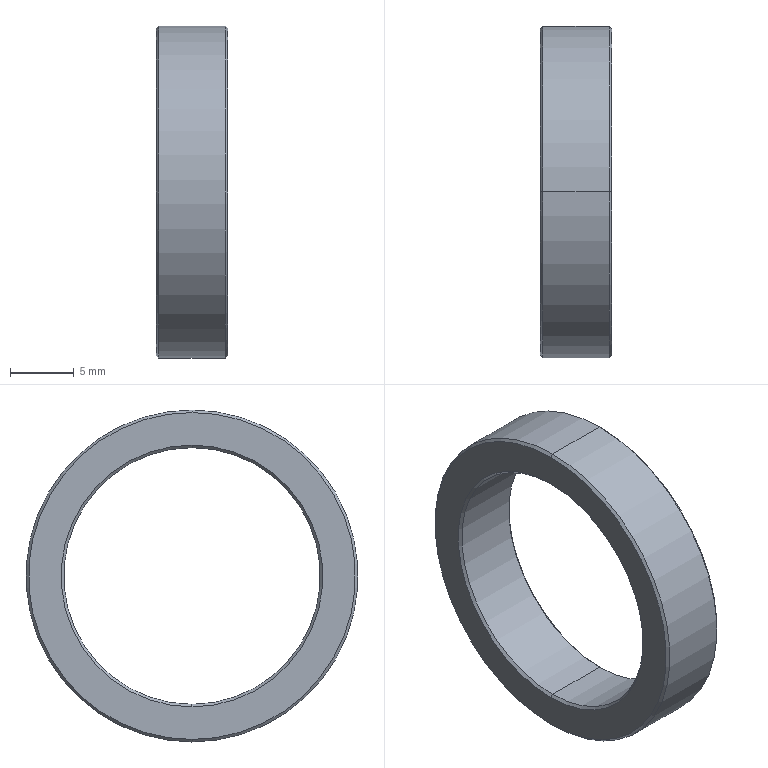Part | STEP file | 1 solid | 14 faces | box 5.6 x 26 x 26 mm | volume 1190 mm3 | cone 8 | cylinder 4 | plane 2 | commonest cylinder face diameters 20.1 x2 26 x2
STEP:
#1=CARTESIAN_POINT('',(0.,0.,0.));
#2=DIRECTION('',(0.,0.,1.));
#3=DIRECTION('',(1.,0.,0.));
#4=AXIS2_PLACEMENT_3D('',#1,#2,#3);
#5=CARTESIAN_POINT('',(0.2,0.,10.05));
#6=VERTEX_POINT('',#5);
#7=CARTESIAN_POINT('',(0.,0.,10.25));
#8=VERTEX_POINT('',#7);
#9=CARTESIAN_POINT('',(0.2,0.,10.05));
#10=DIRECTION('',(-0.7071,0.,0.7071));
#11=VECTOR('',#10,1.);
#12=LINE('',#9,#11);
#13=CARTESIAN_POINT('',(0.2,0.,0.));
#14=DIRECTION('',(-1.,0.,0.));
#15=DIRECTION('',(0.,0.,1.));
#16=AXIS2_PLACEMENT_3D('',#13,#14,#15);
#17=CONICAL_SURFACE('',#16,10.05,0.7854);
#18=CARTESIAN_POINT('',(6.283,0.));
#19=DIRECTION('',(0.,1.));
#20=VECTOR('',#19,1.);
#21=LINE('',#18,#20);
#22=(GEOMETRIC_REPRESENTATION_CONTEXT(2)PARAMETRIC_REPRESENTATION_CONTEXT()REPRESENTATION_CONTEXT('',''));
#23=DEFINITIONAL_REPRESENTATION('',(#21),#22);
#24=PCURVE('',#17,#23);
#25=CARTESIAN_POINT('',(0.2,0.,0.));
#26=DIRECTION('',(-1.,0.,0.));
#27=DIRECTION('',(0.,0.,1.));
#28=AXIS2_PLACEMENT_3D('',#25,#26,#27);
#29=CONICAL_SURFACE('',#28,10.05,0.7854);
#30=CARTESIAN_POINT('',(0.,0.));
#31=DIRECTION('',(0.,1.));
#32=VECTOR('',#31,1.);
#33=LINE('',#30,#32);
#34=(GEOMETRIC_REPRESENTATION_CONTEXT(2)PARAMETRIC_REPRESENTATION_CONTEXT()REPRESENTATION_CONTEXT('',''));
#35=DEFINITIONAL_REPRESENTATION('',(#33),#34);
#36=PCURVE('',#29,#35);
#37=SURFACE_CURVE('',#12,(#24,#36),.PCURVE_S1.);
#38=EDGE_CURVE('',#6,#8,#37,.T.);
#39=ORIENTED_EDGE('',*,*,#38,.T.);
#40=CARTESIAN_POINT('',(0.,0.,-10.25));
#41=VERTEX_POINT('',#40);
#42=CARTESIAN_POINT('',(0.,0.,0.));
#43=DIRECTION('',(1.,0.,0.));
#44=DIRECTION('',(0.,0.,-1.));
#45=AXIS2_PLACEMENT_3D('',#42,#43,#44);
#46=CIRCLE('',#45,10.25);
#47=CARTESIAN_POINT('',(9.425,0.2));
#48=DIRECTION('',(-1.,0.));
#49=VECTOR('',#48,1.);
#50=LINE('',#47,#49);
#51=(GEOMETRIC_REPRESENTATION_CONTEXT(2)PARAMETRIC_REPRESENTATION_CONTEXT()REPRESENTATION_CONTEXT('',''));
#52=DEFINITIONAL_REPRESENTATION('',(#50),#51);
#53=PCURVE('',#17,#52);
#54=CARTESIAN_POINT('',(0.,13.,0.));
#55=DIRECTION('',(1.,0.,0.));
#56=DIRECTION('',(0.,0.,-1.));
#57=AXIS2_PLACEMENT_3D('',#54,#55,#56);
#58=PLANE('',#57);
#59=CARTESIAN_POINT('',(0.,-13.));
#60=DIRECTION('',(1.,0.));
#61=AXIS2_PLACEMENT_2D('',#59,#60);
#62=CIRCLE('',#61,10.25);
#63=(GEOMETRIC_REPRESENTATION_CONTEXT(2)PARAMETRIC_REPRESENTATION_CONTEXT()REPRESENTATION_CONTEXT('',''));
#64=DEFINITIONAL_REPRESENTATION('',(#62),#63);
#65=PCURVE('',#58,#64);
#66=SURFACE_CURVE('',#46,(#53,#65),.PCURVE_S1.);
#67=EDGE_CURVE('',#8,#41,#66,.T.);
#68=ORIENTED_EDGE('',*,*,#67,.T.);
#69=CARTESIAN_POINT('',(0.2,0.,-10.05));
#70=VERTEX_POINT('',#69);
#71=CARTESIAN_POINT('',(0.2,0.,-10.05));
#72=DIRECTION('',(-0.7071,0.,-0.7071));
#73=VECTOR('',#72,1.);
#74=LINE('',#71,#73);
#75=CARTESIAN_POINT('',(3.142,0.));
#76=DIRECTION('',(0.,1.));
#77=VECTOR('',#76,1.);
#78=LINE('',#75,#77);
#79=(GEOMETRIC_REPRESENTATION_CONTEXT(2)PARAMETRIC_REPRESENTATION_CONTEXT()REPRESENTATION_CONTEXT('',''));
#80=DEFINITIONAL_REPRESENTATION('',(#78),#79);
#81=PCURVE('',#17,#80);
#82=CARTESIAN_POINT('',(3.142,0.));
#83=DIRECTION('',(0.,1.));
#84=VECTOR('',#83,1.);
#85=LINE('',#82,#84);
#86=(GEOMETRIC_REPRESENTATION_CONTEXT(2)PARAMETRIC_REPRESENTATION_CONTEXT()REPRESENTATION_CONTEXT('',''));
#87=DEFINITIONAL_REPRESENTATION('',(#85),#86);
#88=PCURVE('',#29,#87);
#89=SURFACE_CURVE('',#74,(#81,#88),.PCURVE_S1.);
#90=EDGE_CURVE('',#70,#41,#89,.T.);
#91=ORIENTED_EDGE('',*,*,#90,.F.);
#92=CARTESIAN_POINT('',(0.2,0.,0.));
#93=DIRECTION('',(-1.,0.,0.));
#94=DIRECTION('',(0.,0.,-1.));
#95=AXIS2_PLACEMENT_3D('',#92,#93,#94);
#96=CIRCLE('',#95,10.05);
#97=CARTESIAN_POINT('',(3.142,0.));
#98=DIRECTION('',(1.,0.));
#99=VECTOR('',#98,1.);
#100=LINE('',#97,#99);
#101=(GEOMETRIC_REPRESENTATION_CONTEXT(2)PARAMETRIC_REPRESENTATION_CONTEXT()REPRESENTATION_CONTEXT('',''));
#102=DEFINITIONAL_REPRESENTATION('',(#100),#101);
#103=PCURVE('',#17,#102);
#104=CARTESIAN_POINT('',(0.,0.,0.));
#105=DIRECTION('',(-1.,0.,0.));
#106=DIRECTION('',(0.,0.,1.));
#107=AXIS2_PLACEMENT_3D('',#104,#105,#106);
#108=CYLINDRICAL_SURFACE('',#107,10.05);
#109=CARTESIAN_POINT('',(3.142,-0.2));
#110=DIRECTION('',(1.,0.));
#111=VECTOR('',#110,1.);
#112=LINE('',#109,#111);
#113=(GEOMETRIC_REPRESENTATION_CONTEXT(2)PARAMETRIC_REPRESENTATION_CONTEXT()REPRESENTATION_CONTEXT('',''));
#114=DEFINITIONAL_REPRESENTATION('',(#112),#113);
#115=PCURVE('',#108,#114);
#116=SURFACE_CURVE('',#96,(#103,#115),.PCURVE_S1.);
#117=EDGE_CURVE('',#70,#6,#116,.T.);
#118=ORIENTED_EDGE('',*,*,#117,.T.);
#119=EDGE_LOOP('',(#39,#68,#91,#118));
#120=FACE_BOUND('',#119,.F.);
#121=ADVANCED_FACE('',(#120),#17,.F.);
#122=CARTESIAN_POINT('',(0.,0.,12.8));
#123=VERTEX_POINT('',#122);
#124=CARTESIAN_POINT('',(0.,0.,-12.8));
#125=VERTEX_POINT('',#124);
#126=CARTESIAN_POINT('',(0.,0.,0.));
#127=DIRECTION('',(-1.,0.,0.));
#128=DIRECTION('',(0.,0.,-1.));
#129=AXIS2_PLACEMENT_3D('',#126,#127,#128);
#130=CIRCLE('',#129,12.8);
#131=CARTESIAN_POINT('',(0.,0.,0.));
#132=DIRECTION('',(1.,0.,0.));
#133=DIRECTION('',(0.,0.,-1.));
#134=AXIS2_PLACEMENT_3D('',#131,#132,#133);
#135=CONICAL_SURFACE('',#134,12.8,0.7854);
#136=CARTESIAN_POINT('',(6.283,0.));
#137=DIRECTION('',(-1.,0.));
#138=VECTOR('',#137,1.);
#139=LINE('',#136,#138);
#140=(GEOMETRIC_REPRESENTATION_CONTEXT(2)PARAMETRIC_REPRESENTATION_CONTEXT()REPRESENTATION_CONTEXT('',''));
#141=DEFINITIONAL_REPRESENTATION('',(#139),#140);
#142=PCURVE('',#135,#141);
#143=CARTESIAN_POINT('',(12.8,-13.));
#144=CARTESIAN_POINT('',(12.8,-35.17));
#145=CARTESIAN_POINT('',(-6.4,-24.085));
#146=CARTESIAN_POINT('',(-25.6,-13.));
#147=CARTESIAN_POINT('',(-6.4,-1.915));
#148=CARTESIAN_POINT('',(12.8,9.17));
#149=CARTESIAN_POINT('',(12.8,-13.));
#150=(BOUNDED_CURVE()B_SPLINE_CURVE(2,(#143,#144,#145,#146,#147,#148,#149),.UNSPECIFIED.,.T.,.F.)B_SPLINE_CURVE_WITH_KNOTS((1,2,2,2,2,1),(-2.094,0.,2.094,4.189,6.283,8.378),.UNSPECIFIED.)CURVE()GEOMETRIC_REPRESENTATION_ITEM()RATIONAL_B_SPLINE_CURVE((1.,0.5,1.,0.5,1.,0.5,1.))REPRESENTATION_ITEM(''));
#151=(GEOMETRIC_REPRESENTATION_CONTEXT(2)PARAMETRIC_REPRESENTATION_CONTEXT()REPRESENTATION_CONTEXT('',''));
#152=DEFINITIONAL_REPRESENTATION('',(#150),#151);
#153=PCURVE('',#58,#152);
#154=SURFACE_CURVE('',#130,(#142,#153),.PCURVE_S1.);
#155=EDGE_CURVE('',#123,#125,#154,.T.);
#156=ORIENTED_EDGE('',*,*,#155,.F.);
#157=CARTESIAN_POINT('',(0.2,0.,13.));
#158=VERTEX_POINT('',#157);
#159=CARTESIAN_POINT('',(0.,0.,12.8));
#160=DIRECTION('',(0.7071,0.,0.7071));
#161=VECTOR('',#160,1.);
#162=LINE('',#159,#161);
#163=CARTESIAN_POINT('',(3.142,0.));
#164=DIRECTION('',(0.,1.));
#165=VECTOR('',#164,1.);
#166=LINE('',#163,#165);
#167=(GEOMETRIC_REPRESENTATION_CONTEXT(2)PARAMETRIC_REPRESENTATION_CONTEXT()REPRESENTATION_CONTEXT('',''));
#168=DEFINITIONAL_REPRESENTATION('',(#166),#167);
#169=PCURVE('',#135,#168);
#170=CARTESIAN_POINT('',(0.,0.,0.));
#171=DIRECTION('',(1.,0.,0.));
#172=DIRECTION('',(0.,0.,-1.));
#173=AXIS2_PLACEMENT_3D('',#170,#171,#172);
#174=CONICAL_SURFACE('',#173,12.8,0.7854);
#175=CARTESIAN_POINT('',(3.142,0.));
#176=DIRECTION('',(0.,1.));
#177=VECTOR('',#176,1.);
#178=LINE('',#175,#177);
#179=(GEOMETRIC_REPRESENTATION_CONTEXT(2)PARAMETRIC_REPRESENTATION_CONTEXT()REPRESENTATION_CONTEXT('',''));
#180=DEFINITIONAL_REPRESENTATION('',(#178),#179);
#181=PCURVE('',#174,#180);
#182=SURFACE_CURVE('',#162,(#169,#181),.PCURVE_S1.);
#183=EDGE_CURVE('',#123,#158,#182,.T.);
#184=ORIENTED_EDGE('',*,*,#183,.T.);
#185=CARTESIAN_POINT('',(0.2,0.,-13.));
#186=VERTEX_POINT('',#185);
#187=CARTESIAN_POINT('',(0.2,0.,0.));
#188=DIRECTION('',(1.,0.,0.));
#189=DIRECTION('',(0.,0.,-1.));
#190=AXIS2_PLACEMENT_3D('',#187,#188,#189);
#191=CIRCLE('',#190,13.);
#192=CARTESIAN_POINT('',(0.,0.2));
#193=DIRECTION('',(1.,0.));
#194=VECTOR('',#193,1.);
#195=LINE('',#192,#194);
#196=(GEOMETRIC_REPRESENTATION_CONTEXT(2)PARAMETRIC_REPRESENTATION_CONTEXT()REPRESENTATION_CONTEXT('',''));
#197=DEFINITIONAL_REPRESENTATION('',(#195),#196);
#198=PCURVE('',#135,#197);
#199=CARTESIAN_POINT('',(0.,0.,0.));
#200=DIRECTION('',(-1.,0.,0.));
#201=DIRECTION('',(0.,0.,1.));
#202=AXIS2_PLACEMENT_3D('',#199,#200,#201);
#203=CYLINDRICAL_SURFACE('',#202,13.);
#204=CARTESIAN_POINT('',(3.142,-0.2));
#205=DIRECTION('',(-1.,0.));
#206=VECTOR('',#205,1.);
#207=LINE('',#204,#206);
#208=(GEOMETRIC_REPRESENTATION_CONTEXT(2)PARAMETRIC_REPRESENTATION_CONTEXT()REPRESENTATION_CONTEXT('',''));
#209=DEFINITIONAL_REPRESENTATION('',(#207),#208);
#210=PCURVE('',#203,#209);
#211=SURFACE_CURVE('',#191,(#198,#210),.PCURVE_S1.);
#212=EDGE_CURVE('',#186,#158,#211,.T.);
#213=ORIENTED_EDGE('',*,*,#212,.F.);
#214=CARTESIAN_POINT('',(0.,0.,-12.8));
#215=DIRECTION('',(0.7071,0.,-0.7071));
#216=VECTOR('',#215,1.);
#217=LINE('',#214,#216);
#218=CARTESIAN_POINT('',(0.,0.));
#219=DIRECTION('',(0.,1.));
#220=VECTOR('',#219,1.);
#221=LINE('',#218,#220);
#222=(GEOMETRIC_REPRESENTATION_CONTEXT(2)PARAMETRIC_REPRESENTATION_CONTEXT()REPRESENTATION_CONTEXT('',''));
#223=DEFINITIONAL_REPRESENTATION('',(#221),#222);
#224=PCURVE('',#135,#223);
#225=CARTESIAN_POINT('',(6.283,0.));
#226=DIRECTION('',(0.,1.));
#227=VECTOR('',#226,1.);
#228=LINE('',#225,#227);
#229=(GEOMETRIC_REPRESENTATION_CONTEXT(2)PARAMETRIC_REPRESENTATION_CONTEXT()REPRESENTATION_CONTEXT('',''));
#230=DEFINITIONAL_REPRESENTATION('',(#228),#229);
#231=PCURVE('',#174,#230);
#232=SURFACE_CURVE('',#217,(#224,#231),.PCURVE_S1.);
#233=EDGE_CURVE('',#125,#186,#232,.T.);
#234=ORIENTED_EDGE('',*,*,#233,.F.);
#235=EDGE_LOOP('',(#156,#184,#213,#234));
#236=FACE_BOUND('',#235,.T.);
#237=ADVANCED_FACE('',(#236),#135,.T.);
#238=CARTESIAN_POINT('',(5.6,0.,-12.8));
#239=VERTEX_POINT('',#238);
#240=CARTESIAN_POINT('',(5.6,0.,12.8));
#241=VERTEX_POINT('',#240);
#242=CARTESIAN_POINT('',(5.6,0.,0.));
#243=DIRECTION('',(1.,0.,0.));
#244=DIRECTION('',(0.,0.,1.));
#245=AXIS2_PLACEMENT_3D('',#242,#243,#244);
#246=CIRCLE('',#245,12.8);
#247=CARTESIAN_POINT('',(5.4,0.,0.));
#248=DIRECTION('',(-1.,0.,0.));
#249=DIRECTION('',(0.,0.,1.));
#250=AXIS2_PLACEMENT_3D('',#247,#248,#249);
#251=CONICAL_SURFACE('',#250,13.,0.7854);
#252=CARTESIAN_POINT('',(6.283,-0.2));
#253=DIRECTION('',(-1.,0.));
#254=VECTOR('',#253,1.);
#255=LINE('',#252,#254);
#256=(GEOMETRIC_REPRESENTATION_CONTEXT(2)PARAMETRIC_REPRESENTATION_CONTEXT()REPRESENTATION_CONTEXT('',''));
#257=DEFINITIONAL_REPRESENTATION('',(#255),#256);
#258=PCURVE('',#251,#257);
#259=CARTESIAN_POINT('',(5.6,13.,0.));
#260=DIRECTION('',(-1.,0.,0.));
#261=DIRECTION('',(0.,0.,1.));
#262=AXIS2_PLACEMENT_3D('',#259,#260,#261);
#263=PLANE('',#262);
#264=CARTESIAN_POINT('',(12.8,-13.));
#265=CARTESIAN_POINT('',(12.8,-35.17));
#266=CARTESIAN_POINT('',(-6.4,-24.085));
#267=CARTESIAN_POINT('',(-25.6,-13.));
#268=CARTESIAN_POINT('',(-6.4,-1.915));
#269=CARTESIAN_POINT('',(12.8,9.17));
#270=CARTESIAN_POINT('',(12.8,-13.));
#271=(BOUNDED_CURVE()B_SPLINE_CURVE(2,(#264,#265,#266,#267,#268,#269,#270),.UNSPECIFIED.,.T.,.F.)B_SPLINE_CURVE_WITH_KNOTS((1,2,2,2,2,1),(-2.094,0.,2.094,4.189,6.283,8.378),.UNSPECIFIED.)CURVE()GEOMETRIC_REPRESENTATION_ITEM()RATIONAL_B_SPLINE_CURVE((1.,0.5,1.,0.5,1.,0.5,1.))REPRESENTATION_ITEM(''));
#272=(GEOMETRIC_REPRESENTATION_CONTEXT(2)PARAMETRIC_REPRESENTATION_CONTEXT()REPRESENTATION_CONTEXT('',''));
#273=DEFINITIONAL_REPRESENTATION('',(#271),#272);
#274=PCURVE('',#263,#273);
#275=SURFACE_CURVE('',#246,(#258,#274),.PCURVE_S1.);
#276=EDGE_CURVE('',#239,#241,#275,.T.);
#277=ORIENTED_EDGE('',*,*,#276,.F.);
#278=CARTESIAN_POINT('',(5.4,0.,-13.));
#279=VERTEX_POINT('',#278);
#280=CARTESIAN_POINT('',(5.4,0.,-13.));
#281=DIRECTION('',(-0.7071,0.,-0.7071));
#282=VECTOR('',#281,1.);
#283=LINE('',#280,#282);
#284=CARTESIAN_POINT('',(3.142,0.));
#285=DIRECTION('',(0.,1.));
#286=VECTOR('',#285,1.);
#287=LINE('',#284,#286);
#288=(GEOMETRIC_REPRESENTATION_CONTEXT(2)PARAMETRIC_REPRESENTATION_CONTEXT()REPRESENTATION_CONTEXT('',''));
#289=DEFINITIONAL_REPRESENTATION('',(#287),#288);
#290=PCURVE('',#251,#289);
#291=CARTESIAN_POINT('',(5.4,0.,0.));
#292=DIRECTION('',(-1.,0.,0.));
#293=DIRECTION('',(0.,0.,1.));
#294=AXIS2_PLACEMENT_3D('',#291,#292,#293);
#295=CONICAL_SURFACE('',#294,13.,0.7854);
#296=CARTESIAN_POINT('',(3.142,0.));
#297=DIRECTION('',(0.,1.));
#298=VECTOR('',#297,1.);
#299=LINE('',#296,#298);
#300=(GEOMETRIC_REPRESENTATION_CONTEXT(2)PARAMETRIC_REPRESENTATION_CONTEXT()REPRESENTATION_CONTEXT('',''));
#301=DEFINITIONAL_REPRESENTATION('',(#299),#300);
#302=PCURVE('',#295,#301);
#303=SURFACE_CURVE('',#283,(#290,#302),.PCURVE_S1.);
#304=EDGE_CURVE('',#239,#279,#303,.T.);
#305=ORIENTED_EDGE('',*,*,#304,.T.);
#306=CARTESIAN_POINT('',(5.4,0.,13.));
#307=VERTEX_POINT('',#306);
#308=CARTESIAN_POINT('',(5.4,0.,0.));
#309=DIRECTION('',(-1.,0.,0.));
#310=DIRECTION('',(0.,0.,1.));
#311=AXIS2_PLACEMENT_3D('',#308,#309,#310);
#312=CIRCLE('',#311,13.);
#313=CARTESIAN_POINT('',(0.,0.));
#314=DIRECTION('',(1.,0.));
#315=VECTOR('',#314,1.);
#316=LINE('',#313,#315);
#317=(GEOMETRIC_REPRESENTATION_CONTEXT(2)PARAMETRIC_REPRESENTATION_CONTEXT()REPRESENTATION_CONTEXT('',''));
#318=DEFINITIONAL_REPRESENTATION('',(#316),#317);
#319=PCURVE('',#251,#318);
#320=CARTESIAN_POINT('',(0.,-5.4));
#321=DIRECTION('',(1.,0.));
#322=VECTOR('',#321,1.);
#323=LINE('',#320,#322);
#324=(GEOMETRIC_REPRESENTATION_CONTEXT(2)PARAMETRIC_REPRESENTATION_CONTEXT()REPRESENTATION_CONTEXT('',''));
#325=DEFINITIONAL_REPRESENTATION('',(#323),#324);
#326=PCURVE('',#203,#325);
#327=SURFACE_CURVE('',#312,(#319,#326),.PCURVE_S1.);
#328=EDGE_CURVE('',#307,#279,#327,.T.);
#329=ORIENTED_EDGE('',*,*,#328,.F.);
#330=CARTESIAN_POINT('',(5.4,0.,13.));
#331=DIRECTION('',(-0.7071,0.,0.7071));
#332=VECTOR('',#331,1.);
#333=LINE('',#330,#332);
#334=CARTESIAN_POINT('',(0.,0.));
#335=DIRECTION('',(0.,1.));
#336=VECTOR('',#335,1.);
#337=LINE('',#334,#336);
#338=(GEOMETRIC_REPRESENTATION_CONTEXT(2)PARAMETRIC_REPRESENTATION_CONTEXT()REPRESENTATION_CONTEXT('',''));
#339=DEFINITIONAL_REPRESENTATION('',(#337),#338);
#340=PCURVE('',#251,#339);
#341=CARTESIAN_POINT('',(6.283,0.));
#342=DIRECTION('',(0.,1.));
#343=VECTOR('',#342,1.);
#344=LINE('',#341,#343);
#345=(GEOMETRIC_REPRESENTATION_CONTEXT(2)PARAMETRIC_REPRESENTATION_CONTEXT()REPRESENTATION_CONTEXT('',''));
#346=DEFINITIONAL_REPRESENTATION('',(#344),#345);
#347=PCURVE('',#295,#346);
#348=SURFACE_CURVE('',#333,(#340,#347),.PCURVE_S1.);
#349=EDGE_CURVE('',#241,#307,#348,.T.);
#350=ORIENTED_EDGE('',*,*,#349,.F.);
#351=EDGE_LOOP('',(#277,#305,#329,#350));
#352=FACE_BOUND('',#351,.T.);
#353=ADVANCED_FACE('',(#352),#251,.T.);
#354=CARTESIAN_POINT('',(5.4,0.,-10.05));
#355=VERTEX_POINT('',#354);
#356=CARTESIAN_POINT('',(5.6,0.,-10.25));
#357=VERTEX_POINT('',#356);
#358=CARTESIAN_POINT('',(5.6,0.,-10.25));
#359=DIRECTION('',(0.7071,0.,-0.7071));
#360=VECTOR('',#359,1.);
#361=LINE('',#358,#360);
#362=CARTESIAN_POINT('',(5.6,0.,0.));
#363=DIRECTION('',(1.,0.,0.));
#364=DIRECTION('',(0.,0.,-1.));
#365=AXIS2_PLACEMENT_3D('',#362,#363,#364);
#366=CONICAL_SURFACE('',#365,10.25,0.7854);
#367=CARTESIAN_POINT('',(6.283,0.));
#368=DIRECTION('',(0.,1.));
#369=VECTOR('',#368,1.);
#370=LINE('',#367,#369);
#371=(GEOMETRIC_REPRESENTATION_CONTEXT(2)PARAMETRIC_REPRESENTATION_CONTEXT()REPRESENTATION_CONTEXT('',''));
#372=DEFINITIONAL_REPRESENTATION('',(#370),#371);
#373=PCURVE('',#366,#372);
#374=CARTESIAN_POINT('',(5.6,0.,0.));
#375=DIRECTION('',(1.,0.,0.));
#376=DIRECTION('',(0.,0.,-1.));
#377=AXIS2_PLACEMENT_3D('',#374,#375,#376);
#378=CONICAL_SURFACE('',#377,10.25,0.7854);
#379=CARTESIAN_POINT('',(0.,0.));
#380=DIRECTION('',(0.,1.));
#381=VECTOR('',#380,1.);
#382=LINE('',#379,#381);
#383=(GEOMETRIC_REPRESENTATION_CONTEXT(2)PARAMETRIC_REPRESENTATION_CONTEXT()REPRESENTATION_CONTEXT('',''));
#384=DEFINITIONAL_REPRESENTATION('',(#382),#383);
#385=PCURVE('',#378,#384);
#386=SURFACE_CURVE('',#361,(#373,#385),.PCURVE_S1.);
#387=EDGE_CURVE('',#355,#357,#386,.T.);
#388=ORIENTED_EDGE('',*,*,#387,.T.);
#389=CARTESIAN_POINT('',(5.6,0.,10.25));
#390=VERTEX_POINT('',#389);
#391=CARTESIAN_POINT('',(5.6,0.,0.));
#392=DIRECTION('',(-1.,0.,0.));
#393=DIRECTION('',(0.,0.,1.));
#394=AXIS2_PLACEMENT_3D('',#391,#392,#393);
#395=CIRCLE('',#394,10.25);
#396=CARTESIAN_POINT('',(9.425,0.));
#397=DIRECTION('',(-1.,0.));
#398=VECTOR('',#397,1.);
#399=LINE('',#396,#398);
#400=(GEOMETRIC_REPRESENTATION_CONTEXT(2)PARAMETRIC_REPRESENTATION_CONTEXT()REPRESENTATION_CONTEXT('',''));
#401=DEFINITIONAL_REPRESENTATION('',(#399),#400);
#402=PCURVE('',#366,#401);
#403=CARTESIAN_POINT('',(0.,-13.));
#404=DIRECTION('',(1.,0.));
#405=AXIS2_PLACEMENT_2D('',#403,#404);
#406=CIRCLE('',#405,10.25);
#407=(GEOMETRIC_REPRESENTATION_CONTEXT(2)PARAMETRIC_REPRESENTATION_CONTEXT()REPRESENTATION_CONTEXT('',''));
#408=DEFINITIONAL_REPRESENTATION('',(#406),#407);
#409=PCURVE('',#263,#408);
#410=SURFACE_CURVE('',#395,(#402,#409),.PCURVE_S1.);
#411=EDGE_CURVE('',#357,#390,#410,.T.);
#412=ORIENTED_EDGE('',*,*,#411,.T.);
#413=CARTESIAN_POINT('',(5.4,0.,10.05));
#414=VERTEX_POINT('',#413);
#415=CARTESIAN_POINT('',(5.6,0.,10.25));
#416=DIRECTION('',(0.7071,0.,0.7071));
#417=VECTOR('',#416,1.);
#418=LINE('',#415,#417);
#419=CARTESIAN_POINT('',(3.142,0.));
#420=DIRECTION('',(0.,1.));
#421=VECTOR('',#420,1.);
#422=LINE('',#419,#421);
#423=(GEOMETRIC_REPRESENTATION_CONTEXT(2)PARAMETRIC_REPRESENTATION_CONTEXT()REPRESENTATION_CONTEXT('',''));
#424=DEFINITIONAL_REPRESENTATION('',(#422),#423);
#425=PCURVE('',#366,#424);
#426=CARTESIAN_POINT('',(3.142,0.));
#427=DIRECTION('',(0.,1.));
#428=VECTOR('',#427,1.);
#429=LINE('',#426,#428);
#430=(GEOMETRIC_REPRESENTATION_CONTEXT(2)PARAMETRIC_REPRESENTATION_CONTEXT()REPRESENTATION_CONTEXT('',''));
#431=DEFINITIONAL_REPRESENTATION('',(#429),#430);
#432=PCURVE('',#378,#431);
#433=SURFACE_CURVE('',#418,(#425,#432),.PCURVE_S1.);
#434=EDGE_CURVE('',#414,#390,#433,.T.);
#435=ORIENTED_EDGE('',*,*,#434,.F.);
#436=CARTESIAN_POINT('',(5.4,0.,0.));
#437=DIRECTION('',(1.,0.,0.));
#438=DIRECTION('',(0.,0.,1.));
#439=AXIS2_PLACEMENT_3D('',#436,#437,#438);
#440=CIRCLE('',#439,10.05);
#441=CARTESIAN_POINT('',(3.142,-0.2));
#442=DIRECTION('',(1.,0.));
#443=VECTOR('',#442,1.);
#444=LINE('',#441,#443);
#445=(GEOMETRIC_REPRESENTATION_CONTEXT(2)PARAMETRIC_REPRESENTATION_CONTEXT()REPRESENTATION_CONTEXT('',''));
#446=DEFINITIONAL_REPRESENTATION('',(#444),#445);
#447=PCURVE('',#366,#446);
#448=CARTESIAN_POINT('',(6.283,-5.4));
#449=DIRECTION('',(-1.,0.));
#450=VECTOR('',#449,1.);
#451=LINE('',#448,#450);
#452=(GEOMETRIC_REPRESENTATION_CONTEXT(2)PARAMETRIC_REPRESENTATION_CONTEXT()REPRESENTATION_CONTEXT('',''));
#453=DEFINITIONAL_REPRESENTATION('',(#451),#452);
#454=PCURVE('',#108,#453);
#455=SURFACE_CURVE('',#440,(#447,#454),.PCURVE_S1.);
#456=EDGE_CURVE('',#414,#355,#455,.T.);
#457=ORIENTED_EDGE('',*,*,#456,.T.);
#458=EDGE_LOOP('',(#388,#412,#435,#457));
#459=FACE_BOUND('',#458,.F.);
#460=ADVANCED_FACE('',(#459),#366,.F.);
#461=ORIENTED_EDGE('',*,*,#328,.T.);
#462=CARTESIAN_POINT('',(0.,0.,-13.));
#463=DIRECTION('',(-1.,0.,0.));
#464=VECTOR('',#463,1.);
#465=LINE('',#462,#464);
#466=CARTESIAN_POINT('',(3.142,0.));
#467=DIRECTION('',(0.,1.));
#468=VECTOR('',#467,1.);
#469=LINE('',#466,#468);
#470=(GEOMETRIC_REPRESENTATION_CONTEXT(2)PARAMETRIC_REPRESENTATION_CONTEXT()REPRESENTATION_CONTEXT('',''));
#471=DEFINITIONAL_REPRESENTATION('',(#469),#470);
#472=PCURVE('',#203,#471);
#473=CARTESIAN_POINT('',(0.,0.,0.));
#474=DIRECTION('',(-1.,0.,0.));
#475=DIRECTION('',(0.,0.,1.));
#476=AXIS2_PLACEMENT_3D('',#473,#474,#475);
#477=CYLINDRICAL_SURFACE('',#476,13.);
#478=CARTESIAN_POINT('',(3.142,0.));
#479=DIRECTION('',(0.,1.));
#480=VECTOR('',#479,1.);
#481=LINE('',#478,#480);
#482=(GEOMETRIC_REPRESENTATION_CONTEXT(2)PARAMETRIC_REPRESENTATION_CONTEXT()REPRESENTATION_CONTEXT('',''));
#483=DEFINITIONAL_REPRESENTATION('',(#481),#482);
#484=PCURVE('',#477,#483);
#485=SURFACE_CURVE('',#465,(#472,#484),.PCURVE_S1.);
#486=EDGE_CURVE('',#279,#186,#485,.T.);
#487=ORIENTED_EDGE('',*,*,#486,.T.);
#488=ORIENTED_EDGE('',*,*,#212,.T.);
#489=CARTESIAN_POINT('',(0.,0.,13.));
#490=DIRECTION('',(-1.,0.,0.));
#491=VECTOR('',#490,1.);
#492=LINE('',#489,#491);
#493=CARTESIAN_POINT('',(0.,0.));
#494=DIRECTION('',(0.,1.));
#495=VECTOR('',#494,1.);
#496=LINE('',#493,#495);
#497=(GEOMETRIC_REPRESENTATION_CONTEXT(2)PARAMETRIC_REPRESENTATION_CONTEXT()REPRESENTATION_CONTEXT('',''));
#498=DEFINITIONAL_REPRESENTATION('',(#496),#497);
#499=PCURVE('',#203,#498);
#500=CARTESIAN_POINT('',(6.283,0.));
#501=DIRECTION('',(0.,1.));
#502=VECTOR('',#501,1.);
#503=LINE('',#500,#502);
#504=(GEOMETRIC_REPRESENTATION_CONTEXT(2)PARAMETRIC_REPRESENTATION_CONTEXT()REPRESENTATION_CONTEXT('',''));
#505=DEFINITIONAL_REPRESENTATION('',(#503),#504);
#506=PCURVE('',#477,#505);
#507=SURFACE_CURVE('',#492,(#499,#506),.PCURVE_S1.);
#508=EDGE_CURVE('',#307,#158,#507,.T.);
#509=ORIENTED_EDGE('',*,*,#508,.F.);
#510=EDGE_LOOP('',(#461,#487,#488,#509));
#511=FACE_BOUND('',#510,.T.);
#512=ADVANCED_FACE('',(#511),#203,.T.);
#513=CARTESIAN_POINT('',(0.,0.,10.05));
#514=DIRECTION('',(-1.,0.,0.));
#515=VECTOR('',#514,1.);
#516=LINE('',#513,#515);
#517=CARTESIAN_POINT('',(6.283,0.));
#518=DIRECTION('',(0.,1.));
#519=VECTOR('',#518,1.);
#520=LINE('',#517,#519);
#521=(GEOMETRIC_REPRESENTATION_CONTEXT(2)PARAMETRIC_REPRESENTATION_CONTEXT()REPRESENTATION_CONTEXT('',''));
#522=DEFINITIONAL_REPRESENTATION('',(#520),#521);
#523=PCURVE('',#108,#522);
#524=CARTESIAN_POINT('',(0.,0.,0.));
#525=DIRECTION('',(-1.,0.,0.));
#526=DIRECTION('',(0.,0.,1.));
#527=AXIS2_PLACEMENT_3D('',#524,#525,#526);
#528=CYLINDRICAL_SURFACE('',#527,10.05);
#529=CARTESIAN_POINT('',(0.,0.));
#530=DIRECTION('',(0.,1.));
#531=VECTOR('',#530,1.);
#532=LINE('',#529,#531);
#533=(GEOMETRIC_REPRESENTATION_CONTEXT(2)PARAMETRIC_REPRESENTATION_CONTEXT()REPRESENTATION_CONTEXT('',''));
#534=DEFINITIONAL_REPRESENTATION('',(#532),#533);
#535=PCURVE('',#528,#534);
#536=SURFACE_CURVE('',#516,(#523,#535),.PCURVE_S1.);
#537=EDGE_CURVE('',#414,#6,#536,.T.);
#538=ORIENTED_EDGE('',*,*,#537,.T.);
#539=ORIENTED_EDGE('',*,*,#117,.F.);
#540=CARTESIAN_POINT('',(0.,0.,-10.05));
#541=DIRECTION('',(-1.,0.,0.));
#542=VECTOR('',#541,1.);
#543=LINE('',#540,#542);
#544=CARTESIAN_POINT('',(3.142,0.));
#545=DIRECTION('',(0.,1.));
#546=VECTOR('',#545,1.);
#547=LINE('',#544,#546);
#548=(GEOMETRIC_REPRESENTATION_CONTEXT(2)PARAMETRIC_REPRESENTATION_CONTEXT()REPRESENTATION_CONTEXT('',''));
#549=DEFINITIONAL_REPRESENTATION('',(#547),#548);
#550=PCURVE('',#108,#549);
#551=CARTESIAN_POINT('',(3.142,0.));
#552=DIRECTION('',(0.,1.));
#553=VECTOR('',#552,1.);
#554=LINE('',#551,#553);
#555=(GEOMETRIC_REPRESENTATION_CONTEXT(2)PARAMETRIC_REPRESENTATION_CONTEXT()REPRESENTATION_CONTEXT('',''));
#556=DEFINITIONAL_REPRESENTATION('',(#554),#555);
#557=PCURVE('',#528,#556);
#558=SURFACE_CURVE('',#543,(#550,#557),.PCURVE_S1.);
#559=EDGE_CURVE('',#355,#70,#558,.T.);
#560=ORIENTED_EDGE('',*,*,#559,.F.);
#561=ORIENTED_EDGE('',*,*,#456,.F.);
#562=EDGE_LOOP('',(#538,#539,#560,#561));
#563=FACE_BOUND('',#562,.F.);
#564=ADVANCED_FACE('',(#563),#108,.F.);
#565=CARTESIAN_POINT('',(0.,0.,0.));
#566=DIRECTION('',(-1.,0.,0.));
#567=DIRECTION('',(0.,0.,-1.));
#568=AXIS2_PLACEMENT_3D('',#565,#566,#567);
#569=CIRCLE('',#568,12.8);
#570=CARTESIAN_POINT('',(12.8,-13.));
#571=CARTESIAN_POINT('',(12.8,-35.17));
#572=CARTESIAN_POINT('',(-6.4,-24.085));
#573=CARTESIAN_POINT('',(-25.6,-13.));
#574=CARTESIAN_POINT('',(-6.4,-1.915));
#575=CARTESIAN_POINT('',(12.8,9.17));
#576=CARTESIAN_POINT('',(12.8,-13.));
#577=(BOUNDED_CURVE()B_SPLINE_CURVE(2,(#570,#571,#572,#573,#574,#575,#576),.UNSPECIFIED.,.T.,.F.)B_SPLINE_CURVE_WITH_KNOTS((1,2,2,2,2,1),(-2.094,0.,2.094,4.189,6.283,8.378),.UNSPECIFIED.)CURVE()GEOMETRIC_REPRESENTATION_ITEM()RATIONAL_B_SPLINE_CURVE((1.,0.5,1.,0.5,1.,0.5,1.))REPRESENTATION_ITEM(''));
#578=(GEOMETRIC_REPRESENTATION_CONTEXT(2)PARAMETRIC_REPRESENTATION_CONTEXT()REPRESENTATION_CONTEXT('',''));
#579=DEFINITIONAL_REPRESENTATION('',(#577),#578);
#580=PCURVE('',#58,#579);
#581=CARTESIAN_POINT('',(6.283,0.));
#582=DIRECTION('',(-1.,0.));
#583=VECTOR('',#582,1.);
#584=LINE('',#581,#583);
#585=(GEOMETRIC_REPRESENTATION_CONTEXT(2)PARAMETRIC_REPRESENTATION_CONTEXT()REPRESENTATION_CONTEXT('',''));
#586=DEFINITIONAL_REPRESENTATION('',(#584),#585);
#587=PCURVE('',#174,#586);
#588=SURFACE_CURVE('',#569,(#580,#587),.PCURVE_S1.);
#589=EDGE_CURVE('',#125,#123,#588,.T.);
#590=ORIENTED_EDGE('',*,*,#589,.T.);
#591=ORIENTED_EDGE('',*,*,#155,.T.);
#592=EDGE_LOOP('',(#590,#591));
#593=FACE_BOUND('',#592,.T.);
#594=ORIENTED_EDGE('',*,*,#67,.T.);
#595=CARTESIAN_POINT('',(0.,0.,0.));
#596=DIRECTION('',(1.,0.,0.));
#597=DIRECTION('',(0.,0.,-1.));
#598=AXIS2_PLACEMENT_3D('',#595,#596,#597);
#599=CIRCLE('',#598,10.25);
#600=CARTESIAN_POINT('',(0.,-13.));
#601=DIRECTION('',(1.,0.));
#602=AXIS2_PLACEMENT_2D('',#600,#601);
#603=CIRCLE('',#602,10.25);
#604=(GEOMETRIC_REPRESENTATION_CONTEXT(2)PARAMETRIC_REPRESENTATION_CONTEXT()REPRESENTATION_CONTEXT('',''));
#605=DEFINITIONAL_REPRESENTATION('',(#603),#604);
#606=PCURVE('',#58,#605);
#607=CARTESIAN_POINT('',(3.142,0.2));
#608=DIRECTION('',(-1.,0.));
#609=VECTOR('',#608,1.);
#610=LINE('',#607,#609);
#611=(GEOMETRIC_REPRESENTATION_CONTEXT(2)PARAMETRIC_REPRESENTATION_CONTEXT()REPRESENTATION_CONTEXT('',''));
#612=DEFINITIONAL_REPRESENTATION('',(#610),#611);
#613=PCURVE('',#29,#612);
#614=SURFACE_CURVE('',#599,(#606,#613),.PCURVE_S1.);
#615=EDGE_CURVE('',#41,#8,#614,.T.);
#616=ORIENTED_EDGE('',*,*,#615,.T.);
#617=EDGE_LOOP('',(#594,#616));
#618=FACE_BOUND('',#617,.T.);
#619=ADVANCED_FACE('',(#593,#618),#58,.F.);
#620=CARTESIAN_POINT('',(0.2,0.,0.));
#621=DIRECTION('',(-1.,0.,0.));
#622=DIRECTION('',(0.,0.,-1.));
#623=AXIS2_PLACEMENT_3D('',#620,#621,#622);
#624=CIRCLE('',#623,10.05);
#625=CARTESIAN_POINT('',(-3.142,-0.2));
#626=DIRECTION('',(1.,0.));
#627=VECTOR('',#626,1.);
#628=LINE('',#625,#627);
#629=(GEOMETRIC_REPRESENTATION_CONTEXT(2)PARAMETRIC_REPRESENTATION_CONTEXT()REPRESENTATION_CONTEXT('',''));
#630=DEFINITIONAL_REPRESENTATION('',(#628),#629);
#631=PCURVE('',#528,#630);
#632=CARTESIAN_POINT('',(-3.142,0.));
#633=DIRECTION('',(1.,0.));
#634=VECTOR('',#633,1.);
#635=LINE('',#632,#634);
#636=(GEOMETRIC_REPRESENTATION_CONTEXT(2)PARAMETRIC_REPRESENTATION_CONTEXT()REPRESENTATION_CONTEXT('',''));
#637=DEFINITIONAL_REPRESENTATION('',(#635),#636);
#638=PCURVE('',#29,#637);
#639=SURFACE_CURVE('',#624,(#631,#638),.PCURVE_S1.);
#640=EDGE_CURVE('',#6,#70,#639,.T.);
#641=ORIENTED_EDGE('',*,*,#640,.F.);
#642=ORIENTED_EDGE('',*,*,#537,.F.);
#643=CARTESIAN_POINT('',(5.4,0.,0.));
#644=DIRECTION('',(1.,0.,0.));
#645=DIRECTION('',(0.,0.,1.));
#646=AXIS2_PLACEMENT_3D('',#643,#644,#645);
#647=CIRCLE('',#646,10.05);
#648=CARTESIAN_POINT('',(6.283,-5.4));
#649=DIRECTION('',(-1.,0.));
#650=VECTOR('',#649,1.);
#651=LINE('',#648,#650);
#652=(GEOMETRIC_REPRESENTATION_CONTEXT(2)PARAMETRIC_REPRESENTATION_CONTEXT()REPRESENTATION_CONTEXT('',''));
#653=DEFINITIONAL_REPRESENTATION('',(#651),#652);
#654=PCURVE('',#528,#653);
#655=CARTESIAN_POINT('',(-3.142,-0.2));
#656=DIRECTION('',(1.,0.));
#657=VECTOR('',#656,1.);
#658=LINE('',#655,#657);
#659=(GEOMETRIC_REPRESENTATION_CONTEXT(2)PARAMETRIC_REPRESENTATION_CONTEXT()REPRESENTATION_CONTEXT('',''));
#660=DEFINITIONAL_REPRESENTATION('',(#658),#659);
#661=PCURVE('',#378,#660);
#662=SURFACE_CURVE('',#647,(#654,#661),.PCURVE_S1.);
#663=EDGE_CURVE('',#355,#414,#662,.T.);
#664=ORIENTED_EDGE('',*,*,#663,.F.);
#665=ORIENTED_EDGE('',*,*,#559,.T.);
#666=EDGE_LOOP('',(#641,#642,#664,#665));
#667=FACE_BOUND('',#666,.F.);
#668=ADVANCED_FACE('',(#667),#528,.F.);
#669=ORIENTED_EDGE('',*,*,#411,.T.);
#670=CARTESIAN_POINT('',(5.6,0.,0.));
#671=DIRECTION('',(-1.,0.,0.));
#672=DIRECTION('',(0.,0.,1.));
#673=AXIS2_PLACEMENT_3D('',#670,#671,#672);
#674=CIRCLE('',#673,10.25);
#675=CARTESIAN_POINT('',(0.,-13.));
#676=DIRECTION('',(1.,0.));
#677=AXIS2_PLACEMENT_2D('',#675,#676);
#678=CIRCLE('',#677,10.25);
#679=(GEOMETRIC_REPRESENTATION_CONTEXT(2)PARAMETRIC_REPRESENTATION_CONTEXT()REPRESENTATION_CONTEXT('',''));
#680=DEFINITIONAL_REPRESENTATION('',(#678),#679);
#681=PCURVE('',#263,#680);
#682=CARTESIAN_POINT('',(3.142,0.));
#683=DIRECTION('',(-1.,0.));
#684=VECTOR('',#683,1.);
#685=LINE('',#682,#684);
#686=(GEOMETRIC_REPRESENTATION_CONTEXT(2)PARAMETRIC_REPRESENTATION_CONTEXT()REPRESENTATION_CONTEXT('',''));
#687=DEFINITIONAL_REPRESENTATION('',(#685),#686);
#688=PCURVE('',#378,#687);
#689=SURFACE_CURVE('',#674,(#681,#688),.PCURVE_S1.);
#690=EDGE_CURVE('',#390,#357,#689,.T.);
#691=ORIENTED_EDGE('',*,*,#690,.T.);
#692=EDGE_LOOP('',(#669,#691));
#693=FACE_BOUND('',#692,.T.);
#694=CARTESIAN_POINT('',(5.6,0.,0.));
#695=DIRECTION('',(1.,0.,0.));
#696=DIRECTION('',(0.,0.,1.));
#697=AXIS2_PLACEMENT_3D('',#694,#695,#696);
#698=CIRCLE('',#697,12.8);
#699=CARTESIAN_POINT('',(12.8,-13.));
#700=CARTESIAN_POINT('',(12.8,-35.17));
#701=CARTESIAN_POINT('',(-6.4,-24.085));
#702=CARTESIAN_POINT('',(-25.6,-13.));
#703=CARTESIAN_POINT('',(-6.4,-1.915));
#704=CARTESIAN_POINT('',(12.8,9.17));
#705=CARTESIAN_POINT('',(12.8,-13.));
#706=(BOUNDED_CURVE()B_SPLINE_CURVE(2,(#699,#700,#701,#702,#703,#704,#705),.UNSPECIFIED.,.T.,.F.)B_SPLINE_CURVE_WITH_KNOTS((1,2,2,2,2,1),(-2.094,0.,2.094,4.189,6.283,8.378),.UNSPECIFIED.)CURVE()GEOMETRIC_REPRESENTATION_ITEM()RATIONAL_B_SPLINE_CURVE((1.,0.5,1.,0.5,1.,0.5,1.))REPRESENTATION_ITEM(''));
#707=(GEOMETRIC_REPRESENTATION_CONTEXT(2)PARAMETRIC_REPRESENTATION_CONTEXT()REPRESENTATION_CONTEXT('',''));
#708=DEFINITIONAL_REPRESENTATION('',(#706),#707);
#709=PCURVE('',#263,#708);
#710=CARTESIAN_POINT('',(6.283,-0.2));
#711=DIRECTION('',(-1.,0.));
#712=VECTOR('',#711,1.);
#713=LINE('',#710,#712);
#714=(GEOMETRIC_REPRESENTATION_CONTEXT(2)PARAMETRIC_REPRESENTATION_CONTEXT()REPRESENTATION_CONTEXT('',''));
#715=DEFINITIONAL_REPRESENTATION('',(#713),#714);
#716=PCURVE('',#295,#715);
#717=SURFACE_CURVE('',#698,(#709,#716),.PCURVE_S1.);
#718=EDGE_CURVE('',#241,#239,#717,.T.);
#719=ORIENTED_EDGE('',*,*,#718,.T.);
#720=ORIENTED_EDGE('',*,*,#276,.T.);
#721=EDGE_LOOP('',(#719,#720));
#722=FACE_BOUND('',#721,.T.);
#723=ADVANCED_FACE('',(#693,#722),#263,.F.);
#724=ORIENTED_EDGE('',*,*,#486,.F.);
#725=CARTESIAN_POINT('',(5.4,0.,0.));
#726=DIRECTION('',(-1.,0.,0.));
#727=DIRECTION('',(0.,0.,1.));
#728=AXIS2_PLACEMENT_3D('',#725,#726,#727);
#729=CIRCLE('',#728,13.);
#730=CARTESIAN_POINT('',(0.,-5.4));
#731=DIRECTION('',(1.,0.));
#732=VECTOR('',#731,1.);
#733=LINE('',#730,#732);
#734=(GEOMETRIC_REPRESENTATION_CONTEXT(2)PARAMETRIC_REPRESENTATION_CONTEXT()REPRESENTATION_CONTEXT('',''));
#735=DEFINITIONAL_REPRESENTATION('',(#733),#734);
#736=PCURVE('',#477,#735);
#737=CARTESIAN_POINT('',(0.,0.));
#738=DIRECTION('',(1.,0.));
#739=VECTOR('',#738,1.);
#740=LINE('',#737,#739);
#741=(GEOMETRIC_REPRESENTATION_CONTEXT(2)PARAMETRIC_REPRESENTATION_CONTEXT()REPRESENTATION_CONTEXT('',''));
#742=DEFINITIONAL_REPRESENTATION('',(#740),#741);
#743=PCURVE('',#295,#742);
#744=SURFACE_CURVE('',#729,(#736,#743),.PCURVE_S1.);
#745=EDGE_CURVE('',#279,#307,#744,.T.);
#746=ORIENTED_EDGE('',*,*,#745,.T.);
#747=ORIENTED_EDGE('',*,*,#508,.T.);
#748=CARTESIAN_POINT('',(0.2,0.,0.));
#749=DIRECTION('',(1.,0.,0.));
#750=DIRECTION('',(0.,0.,-1.));
#751=AXIS2_PLACEMENT_3D('',#748,#749,#750);
#752=CIRCLE('',#751,13.);
#753=CARTESIAN_POINT('',(9.425,-0.2));
#754=DIRECTION('',(-1.,0.));
#755=VECTOR('',#754,1.);
#756=LINE('',#753,#755);
#757=(GEOMETRIC_REPRESENTATION_CONTEXT(2)PARAMETRIC_REPRESENTATION_CONTEXT()REPRESENTATION_CONTEXT('',''));
#758=DEFINITIONAL_REPRESENTATION('',(#756),#757);
#759=PCURVE('',#477,#758);
#760=CARTESIAN_POINT('',(0.,0.2));
#761=DIRECTION('',(1.,0.));
#762=VECTOR('',#761,1.);
#763=LINE('',#760,#762);
#764=(GEOMETRIC_REPRESENTATION_CONTEXT(2)PARAMETRIC_REPRESENTATION_CONTEXT()REPRESENTATION_CONTEXT('',''));
#765=DEFINITIONAL_REPRESENTATION('',(#763),#764);
#766=PCURVE('',#174,#765);
#767=SURFACE_CURVE('',#752,(#759,#766),.PCURVE_S1.);
#768=EDGE_CURVE('',#158,#186,#767,.T.);
#769=ORIENTED_EDGE('',*,*,#768,.T.);
#770=EDGE_LOOP('',(#724,#746,#747,#769));
#771=FACE_BOUND('',#770,.T.);
#772=ADVANCED_FACE('',(#771),#477,.T.);
#773=ORIENTED_EDGE('',*,*,#690,.T.);
#774=ORIENTED_EDGE('',*,*,#387,.F.);
#775=ORIENTED_EDGE('',*,*,#663,.T.);
#776=ORIENTED_EDGE('',*,*,#434,.T.);
#777=EDGE_LOOP('',(#773,#774,#775,#776));
#778=FACE_BOUND('',#777,.F.);
#779=ADVANCED_FACE('',(#778),#378,.F.);
#780=ORIENTED_EDGE('',*,*,#304,.F.);
#781=ORIENTED_EDGE('',*,*,#718,.F.);
#782=ORIENTED_EDGE('',*,*,#349,.T.);
#783=ORIENTED_EDGE('',*,*,#745,.F.);
#784=EDGE_LOOP('',(#780,#781,#782,#783));
#785=FACE_BOUND('',#784,.T.);
#786=ADVANCED_FACE('',(#785),#295,.T.);
#787=ORIENTED_EDGE('',*,*,#183,.F.);
#788=ORIENTED_EDGE('',*,*,#589,.F.);
#789=ORIENTED_EDGE('',*,*,#233,.T.);
#790=ORIENTED_EDGE('',*,*,#768,.F.);
#791=EDGE_LOOP('',(#787,#788,#789,#790));
#792=FACE_BOUND('',#791,.T.);
#793=ADVANCED_FACE('',(#792),#174,.T.);
#794=ORIENTED_EDGE('',*,*,#615,.T.);
#795=ORIENTED_EDGE('',*,*,#38,.F.);
#796=ORIENTED_EDGE('',*,*,#640,.T.);
#797=ORIENTED_EDGE('',*,*,#90,.T.);
#798=EDGE_LOOP('',(#794,#795,#796,#797));
#799=FACE_BOUND('',#798,.F.);
#800=ADVANCED_FACE('',(#799),#29,.F.);
#801=CLOSED_SHELL('',(#121,#237,#353,#460,#512,#564,#619,#668,#723,#772,#779,#786,#793,#800));
#802=MANIFOLD_SOLID_BREP('',#801);
#803=(LENGTH_UNIT()NAMED_UNIT(*)SI_UNIT(.MILLI.,.METRE.));
#804=UNCERTAINTY_MEASURE_WITH_UNIT(LENGTH_MEASURE(0.0000001),#803,'','');
#805=(NAMED_UNIT(*)PLANE_ANGLE_UNIT()SI_UNIT($,.RADIAN.));
#806=(NAMED_UNIT(*)SI_UNIT($,.STERADIAN.)SOLID_ANGLE_UNIT());
#807=(GEOMETRIC_REPRESENTATION_CONTEXT(3)GLOBAL_UNCERTAINTY_ASSIGNED_CONTEXT((#804))GLOBAL_UNIT_ASSIGNED_CONTEXT((#803,#805,#806))REPRESENTATION_CONTEXT('',''));
#808=ADVANCED_BREP_SHAPE_REPRESENTATION('',(#4,#802),#807);